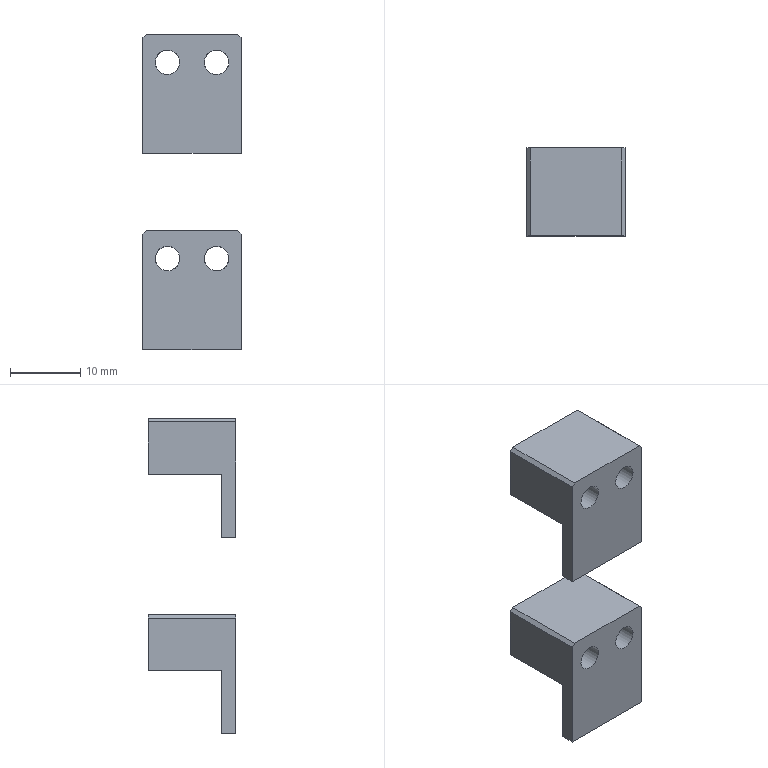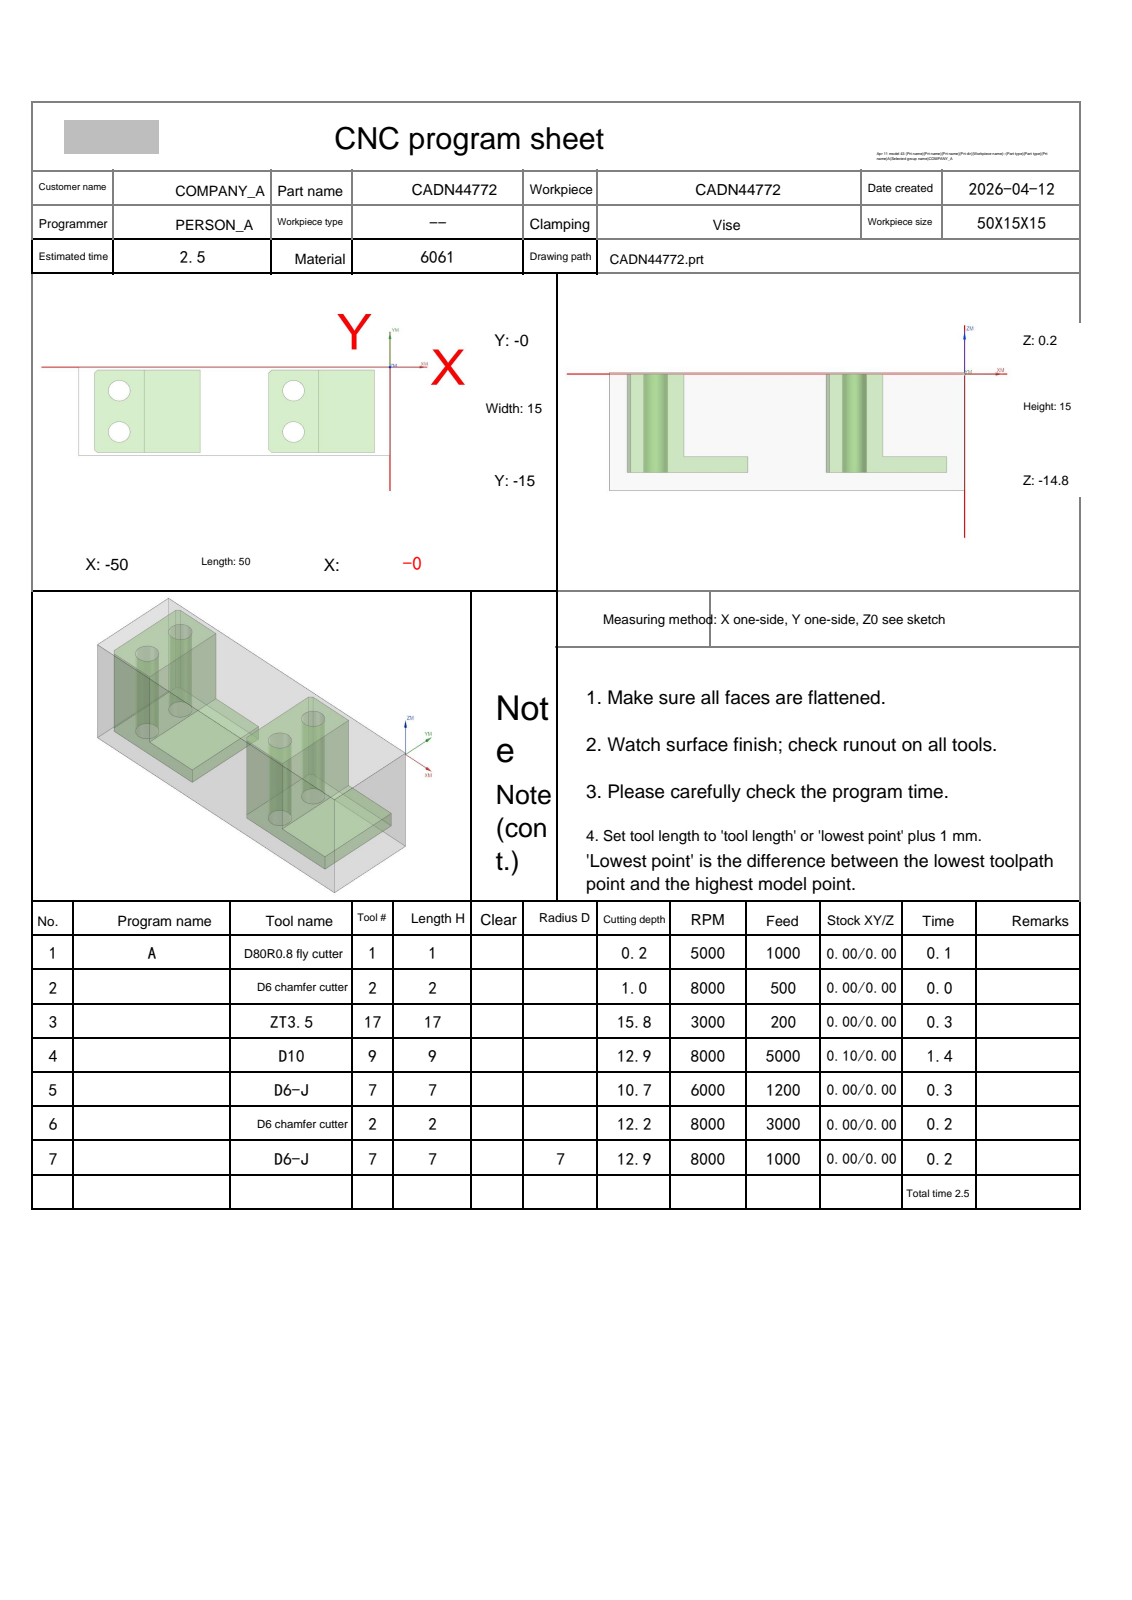NC program | NX | posted by the shop | part box 14 x 12.5 x 45 mm
Whole program:
%
O0001
(Machine time: 3.88 MIN)
(===Total Tool:5===)
(T1=D80R0.8 fly cutter D=80.  R=0.8  D-  H01 Z=-0.   )
(T2=D6 chamfer cutter   D=6.   R=0.   D-  H02 Z=-12.  )
(T17=ZT3.5  D=3.5  DR_a=118 D-  H17 Z=-15.55)
(T9=D10     D=10.  R=0.   D-  H09 Z=-12.7 )
(T7=D6-J    D=6.   R=0.   D7  H07 Z=-12.7 )
G80 G90 G17 G49 G40
G91 G28 Z0
M01
N1 T01 M06
(D80R0.8 fly cutter  D=80. R=0.8 H=01 ce=0.00 di=0.00)
G00 G90 G54 X-92.5 Y-7.5 M03 S5000
G43 H01 Z20.
M08
Z2.
G01 Z0.0 F1000.
X-87.5
X37.5
X42.5
Z2.
G00 Z20.
G91 G28 Z0.0
M05
M09
G91 G28 Z0.0
M01
N2 T02 M06
(D6 chamfer cutter  D=6. R=0. H=02 ce=0.00 di=0.00)
G00 G90 G54 X-43.5 Y-4. M03 S8000
G43 H02 Z20.
M08
G98 G81 X-43.5 Y-4. Z-.8 R1. F500.
Y-11.
X-15.5
Y-4.
G80
G00 Z20.
G91 G28 Z0.0
M05
M09
G91 G28 Z0.0
M01
N3 T17 M06
(ZT3.5 D=3.5 DR_a=118 H=17)
G00 G90 G54 X-43.5 Y-4. M03 S3000
G43 H17 Z20.
M08
G98 G83 X-43.5 Y-4. Z-15.552 R1. F200. Q3.
Y-11.
X-15.5
Y-4.
G80
G00 Z20.
G91 G28 Z0.0
M05
M09
G91 G28 Z0.0
M01
N4 T09 M06
(D10  D=10. R=0. H=09 ce=0.10 di=0.00)
G00 G90 G54 X-10.75 Y4.6 M03 S8000
G43 H09 Z20.
M08
Z.5
G01 X-2.5 Z.431 F5000.
G02 X2.6 Y-.5 Z.365 I0.0 J-5.1
G01 Y-14.5 Z.249
G02 X-2.5 Y-19.6 Z.182 I-5.1 J0.0
G01 X-19. Z.045
G02 X-22.606 Y-18.106 Z.012 I0.0 J5.1
G01 X-23.106 Y-17.606 Z.006
G02 X-24.6 Y-14. Z-.027 I3.606 J3.606
G01 Y-1. Z-.135
G02 X-23.106 Y2.606 Z-.169 I5.1 J0.0
G01 X-22.606 Y3.106 Z-.175
G02 X-19. Y4.6 Z-.208 I3.606 J-3.606
G01 X-2.5 Z-.345
G02 X2.6 Y-.5 Z-.412 I0.0 J-5.1
G01 Y-14.5 Z-.528
G02 X-2.5 Y-19.6 Z-.594 I-5.1 J0.0
G01 X-19. Z-.732
G02 X-22.606 Y-18.106 Z-.765 I0.0 J5.1
G01 X-23.106 Y-17.606 Z-.771
G02 X-24.6 Y-14. Z-.804 I3.606 J3.606
G01 Y-1. Z-.912
G02 X-23.106 Y2.606 Z-.945 I5.1 J0.0
G01 X-22.606 Y3.106 Z-.951
G02 X-19. Y4.6 Z-.984 I3.606 J-3.606
G01 X-2.5 Z-1.121
G02 X2.6 Y-.5 Z-1.188 I0.0 J-5.1
G01 Y-14.5 Z-1.304
G02 X-2.5 Y-19.6 Z-1.371 I-5.1 J0.0
G01 X-19. Z-1.508
G02 X-22.606 Y-18.106 Z-1.541 I0.0 J5.1
G01 X-23.106 Y-17.606 Z-1.547
G02 X-24.6 Y-14. Z-1.58 I3.606 J3.606
G01 Y-1. Z-1.688
G02 X-23.106 Y2.606 Z-1.722 I5.1 J0.0
G01 X-22.606 Y3.106 Z-1.728
G02 X-19. Y4.6 Z-1.761 I3.606 J-3.606
G01 X-2.5 Z-1.898
G02 X2.6 Y-.5 Z-1.965 I0.0 J-5.1
G01 Y-14.5 Z-2.081
G02 X-2.5 Y-19.6 Z-2.147 I-5.1 J0.0
G01 X-19. Z-2.284
G02 X-22.606 Y-18.106 Z-2.318 I0.0 J5.1
G01 X-23.106 Y-17.606 Z-2.324
G02 X-24.6 Y-14. Z-2.357 I3.606 J3.606
G01 Y-1. Z-2.465
G02 X-23.106 Y2.606 Z-2.498 I5.1 J0.0
G01 X-22.606 Y3.106 Z-2.504
G02 X-19. Y4.6 Z-2.537 I3.606 J-3.606
G01 X-2.5 Z-2.674
G02 X2.6 Y-.5 Z-2.741 I0.0 J-5.1
G01 Y-14.5 Z-2.857
G02 X-2.5 Y-19.6 Z-2.924 I-5.1 J0.0
G01 X-19. Z-3.061
G02 X-22.606 Y-18.106 Z-3.094 I0.0 J5.1
G01 X-23.106 Y-17.606 Z-3.1
G02 X-24.6 Y-14. Z-3.133 I3.606 J3.606
G01 Y-1. Z-3.241
G02 X-23.106 Y2.606 Z-3.275 I5.1 J0.0
G01 X-22.606 Y3.106 Z-3.281
G02 X-19. Y4.6 Z-3.314 I3.606 J-3.606
G01 X-2.5 Z-3.451
G02 X2.6 Y-.5 Z-3.517 I0.0 J-5.1
G01 Y-14.5 Z-3.634
G02 X-2.5 Y-19.6 Z-3.7 I-5.1 J0.0
G01 X-19. Z-3.837
G02 X-22.606 Y-18.106 Z-3.871 I0.0 J5.1
G01 X-23.106 Y-17.606 Z-3.877
G02 X-24.6 Y-14. Z-3.91 I3.606 J3.606
G01 Y-1. Z-4.018
G02 X-23.106 Y2.606 Z-4.051 I5.1 J0.0
G01 X-22.606 Y3.106 Z-4.057
G02 X-19. Y4.6 Z-4.09 I3.606 J-3.606
G01 X-2.5 Z-4.227
G02 X2.6 Y-.5 Z-4.294 I0.0 J-5.1
G01 Y-14.5 Z-4.41
G02 X-2.5 Y-19.6 Z-4.477 I-5.1 J0.0
G01 X-19. Z-4.614
G02 X-22.606 Y-18.106 Z-4.647 I0.0 J5.1
G01 X-23.106 Y-17.606 Z-4.653
G02 X-24.6 Y-14. Z-4.686 I3.606 J3.606
G01 Y-1. Z-4.794
G02 X-23.106 Y2.606 Z-4.828 I5.1 J0.0
G01 X-22.606 Y3.106 Z-4.833
G02 X-19. Y4.6 Z-4.867 I3.606 J-3.606
G01 X-2.5 Z-5.004
G02 X2.6 Y-.5 Z-5.07 I0.0 J-5.1
G01 Y-14.5 Z-5.187
G02 X-2.5 Y-19.6 Z-5.253 I-5.1 J0.0
G01 X-19. Z-5.39
G02 X-22.606 Y-18.106 Z-5.424 I0.0 J5.1
G01 X-23.106 Y-17.606 Z-5.43
G02 X-24.6 Y-14. Z-5.463 I3.606 J3.606
G01 Y-1. Z-5.571
G02 X-23.106 Y2.606 Z-5.604 I5.1 J0.0
G01 X-22.606 Y3.106 Z-5.61
G02 X-19. Y4.6 Z-5.643 I3.606 J-3.606
G01 X-2.5 Z-5.78
G02 X2.6 Y-.5 Z-5.847 I0.0 J-5.1
G01 Y-14.5 Z-5.963
G02 X-2.5 Y-19.6 Z-6.03 I-5.1 J0.0
G01 X-19. Z-6.167
G02 X-22.606 Y-18.106 Z-6.2 I0.0 J5.1
G01 X-23.106 Y-17.606 Z-6.206
G02 X-24.6 Y-14. Z-6.239 I3.606 J3.606
G01 Y-1. Z-6.347
G02 X-23.106 Y2.606 Z-6.381 I5.1 J0.0
G01 X-22.606 Y3.106 Z-6.386
G02 X-19. Y4.6 Z-6.42 I3.606 J-3.606
G01 X-2.5 Z-6.557
G02 X2.6 Y-.5 Z-6.623 I0.0 J-5.1
G01 Y-14.5 Z-6.74
G02 X-2.5 Y-19.6 Z-6.806 I-5.1 J0.0
G01 X-19. Z-6.943
G02 X-22.606 Y-18.106 Z-6.977 I0.0 J5.1
G01 X-23.106 Y-17.606 Z-6.982
G02 X-24.6 Y-14. Z-7.016 I3.606 J3.606
G01 Y-1. Z-7.124
G02 X-23.106 Y2.606 Z-7.157 I5.1 J0.0
G01 X-22.606 Y3.106 Z-7.163
G02 X-19. Y4.6 Z-7.196 I3.606 J-3.606
G01 X-2.5 Z-7.333
G02 X2.6 Y-.5 Z-7.4 I0.0 J-5.1
G01 Y-14.5 Z-7.516
G02 X-2.5 Y-19.6 Z-7.583 I-5.1 J0.0
G01 X-19. Z-7.72
G02 X-22.606 Y-18.106 Z-7.753 I0.0 J5.1
G01 X-23.106 Y-17.606 Z-7.759
G02 X-24.6 Y-14. Z-7.792 I3.606 J3.606
G01 Y-1. Z-7.9
G02 X-23.106 Y2.606 Z-7.933 I5.1 J0.0
G01 X-22.606 Y3.106 Z-7.939
G02 X-19. Y4.6 Z-7.973 I3.606 J-3.606
G01 X-2.5 Z-8.11
G02 X2.6 Y-.5 Z-8.176 I0.0 J-5.1
G01 Y-14.5 Z-8.293
G02 X-2.5 Y-19.6 Z-8.359 I-5.1 J0.0
G01 X-19. Z-8.496
G02 X-22.606 Y-18.106 Z-8.53 I0.0 J5.1
G01 X-23.106 Y-17.606 Z-8.535
G02 X-24.6 Y-14. Z-8.569 I3.606 J3.606
G01 Y-1. Z-8.677
G02 X-23.106 Y2.606 Z-8.71 I5.1 J0.0
G01 X-22.606 Y3.106 Z-8.716
G02 X-19. Y4.6 Z-8.749 I3.606 J-3.606
G01 X-2.5 Z-8.886
G02 X2.6 Y-.5 Z-8.953 I0.0 J-5.1
G01 Y-14.5 Z-9.069
G02 X-2.5 Y-19.6 Z-9.136 I-5.1 J0.0
G01 X-19. Z-9.273
G02 X-22.606 Y-18.106 Z-9.306 I0.0 J5.1
G01 X-23.106 Y-17.606 Z-9.312
G02 X-24.6 Y-14. Z-9.345 I3.606 J3.606
G01 Y-1. Z-9.453
G02 X-23.106 Y2.606 Z-9.486 I5.1 J0.0
G01 X-22.606 Y3.106 Z-9.492
G02 X-19. Y4.6 Z-9.526 I3.606 J-3.606
G01 X-2.5 Z-9.663
G02 X2.6 Y-.5 Z-9.729 I0.0 J-5.1
G01 Y-14.5 Z-9.846
G02 X-2.5 Y-19.6 Z-9.912 I-5.1 J0.0
G01 X-19. Z-10.049
G02 X-22.606 Y-18.106 Z-10.082 I0.0 J5.1
G01 X-23.106 Y-17.606 Z-10.088
G02 X-24.6 Y-14. Z-10.122 I3.606 J3.606
G01 Y-1. Z-10.23
G02 X-23.106 Y2.606 Z-10.263 I5.1 J0.0
G01 X-22.606 Y3.106 Z-10.269
G02 X-19. Y4.6 Z-10.302 I3.606 J-3.606
G01 X-2.5 Z-10.439
G02 X2.6 Y-.5 Z-10.506 I0.0 J-5.1
G01 Y-14.5 Z-10.622
G02 X-2.5 Y-19.6 Z-10.689 I-5.1 J0.0
G01 X-19. Z-10.826
G02 X-22.606 Y-18.106 Z-10.859 I0.0 J5.1
G01 X-23.106 Y-17.606 Z-10.865
G02 X-24.6 Y-14. Z-10.898 I3.606 J3.606
G01 Y-1. Z-11.006
G02 X-23.106 Y2.606 Z-11.039 I5.1 J0.0
G01 X-22.606 Y3.106 Z-11.045
G02 X-19. Y4.6 Z-11.079 I3.606 J-3.606
G01 X-2.5 Z-11.216
G02 X2.6 Y-.5 Z-11.282 I0.0 J-5.1
G01 Y-14.5 Z-11.398
G02 X-2.5 Y-19.6 Z-11.465 I-5.1 J0.0
G01 X-19. Z-11.602
G02 X-22.606 Y-18.106 Z-11.635 I0.0 J5.1
G01 X-23.106 Y-17.606 Z-11.641
G02 X-24.6 Y-14. Z-11.675 I3.606 J3.606
G01 Y-1. Z-11.783
G02 X-23.106 Y2.606 Z-11.816 I5.1 J0.0
G01 X-22.606 Y3.106 Z-11.822
G02 X-19. Y4.6 Z-11.855 I3.606 J-3.606
G01 X-2.5 Z-11.992
G02 X2.6 Y-.5 Z-12.059 I0.0 J-5.1
G01 Y-14.5 Z-12.175
G02 X-2.5 Y-19.6 Z-12.242 I-5.1 J0.0
G01 X-19. Z-12.379
G02 X-22.606 Y-18.106 Z-12.412 I0.0 J5.1
G01 X-23.106 Y-17.606 Z-12.418
G02 X-24.6 Y-14. Z-12.451 I3.606 J3.606
G01 Y-1. Z-12.559
G02 X-23.106 Y2.606 Z-12.592 I5.1 J0.0
G01 X-22.606 Y3.106 Z-12.598
G02 X-19. Y4.6 Z-12.631 I3.606 J-3.606
G01 X-10.75 Z-12.7
X-2.5
G02 X2.6 Y-.5 I0.0 J-5.1
G01 Y-14.5
G02 X-2.5 Y-19.6 I-5.1 J0.0
G01 X-19.
G02 X-22.606 Y-18.106 I0.0 J5.1
G01 X-23.106 Y-17.606
G02 X-24.6 Y-14. I3.606 J3.606
G01 Y-1.
G02 X-23.106 Y2.606 I5.1 J0.0
G01 X-22.606 Y3.106
G02 X-19. Y4.6 I3.606 J-3.606
G01 X-10.75
X-10.25
Z-11.7
G00 Z20.
X-38.75
Z.5
G01 X-30.5 Z.431
G02 X-25.4 Y-.5 Z.365 I0.0 J-5.1
G01 Y-14.5 Z.249
G02 X-30.5 Y-19.6 Z.182 I-5.1 J0.0
G01 X-47. Z.045
G02 X-50.606 Y-18.106 Z.012 I0.0 J5.1
G01 X-51.106 Y-17.606 Z.006
G02 X-52.6 Y-14. Z-.027 I3.606 J3.606
G01 Y-1. Z-.135
G02 X-51.106 Y2.606 Z-.169 I5.1 J0.0
G01 X-50.606 Y3.106 Z-.175
G02 X-47. Y4.6 Z-.208 I3.606 J-3.606
G01 X-30.5 Z-.345
G02 X-25.4 Y-.5 Z-.412 I0.0 J-5.1
G01 Y-14.5 Z-.528
G02 X-30.5 Y-19.6 Z-.594 I-5.1 J0.0
G01 X-47. Z-.732
G02 X-50.606 Y-18.106 Z-.765 I0.0 J5.1
G01 X-51.106 Y-17.606 Z-.771
G02 X-52.6 Y-14. Z-.804 I3.606 J3.606
G01 Y-1. Z-.912
G02 X-51.106 Y2.606 Z-.945 I5.1 J0.0
G01 X-50.606 Y3.106 Z-.951
G02 X-47. Y4.6 Z-.984 I3.606 J-3.606
G01 X-30.5 Z-1.121
G02 X-25.4 Y-.5 Z-1.188 I0.0 J-5.1
G01 Y-14.5 Z-1.304
G02 X-30.5 Y-19.6 Z-1.371 I-5.1 J0.0
G01 X-47. Z-1.508
G02 X-50.606 Y-18.106 Z-1.541 I0.0 J5.1
G01 X-51.106 Y-17.606 Z-1.547
G02 X-52.6 Y-14. Z-1.58 I3.606 J3.606
G01 Y-1. Z-1.688
G02 X-51.106 Y2.606 Z-1.722 I5.1 J0.0
G01 X-50.606 Y3.106 Z-1.728
G02 X-47. Y4.6 Z-1.761 I3.606 J-3.606
G01 X-30.5 Z-1.898
G02 X-25.4 Y-.5 Z-1.965 I0.0 J-5.1
G01 Y-14.5 Z-2.081
G02 X-30.5 Y-19.6 Z-2.147 I-5.1 J0.0
G01 X-47. Z-2.284
G02 X-50.606 Y-18.106 Z-2.318 I0.0 J5.1
G01 X-51.106 Y-17.606 Z-2.324
G02 X-52.6 Y-14. Z-2.357 I3.606 J3.606
G01 Y-1. Z-2.465
G02 X-51.106 Y2.606 Z-2.498 I5.1 J0.0
G01 X-50.606 Y3.106 Z-2.504
G02 X-47. Y4.6 Z-2.537 I3.606 J-3.606
G01 X-30.5 Z-2.674
G02 X-25.4 Y-.5 Z-2.741 I0.0 J-5.1
G01 Y-14.5 Z-2.857
G02 X-30.5 Y-19.6 Z-2.924 I-5.1 J0.0
G01 X-47. Z-3.061
G02 X-50.606 Y-18.106 Z-3.094 I0.0 J5.1
G01 X-51.106 Y-17.606 Z-3.1
G02 X-52.6 Y-14. Z-3.133 I3.606 J3.606
G01 Y-1. Z-3.241
G02 X-51.106 Y2.606 Z-3.275 I5.1 J0.0
G01 X-50.606 Y3.106 Z-3.281
G02 X-47. Y4.6 Z-3.314 I3.606 J-3.606
G01 X-30.5 Z-3.451
G02 X-25.4 Y-.5 Z-3.517 I0.0 J-5.1
G01 Y-14.5 Z-3.634
G02 X-30.5 Y-19.6 Z-3.7 I-5.1 J0.0
G01 X-47. Z-3.837
G02 X-50.606 Y-18.106 Z-3.871 I0.0 J5.1
G01 X-51.106 Y-17.606 Z-3.877
G02 X-52.6 Y-14. Z-3.91 I3.606 J3.606
G01 Y-1. Z-4.018
G02 X-51.106 Y2.606 Z-4.051 I5.1 J0.0
G01 X-50.606 Y3.106 Z-4.057
G02 X-47. Y4.6 Z-4.09 I3.606 J-3.606
G01 X-30.5 Z-4.227
G02 X-25.4 Y-.5 Z-4.294 I0.0 J-5.1
G01 Y-14.5 Z-4.41
G02 X-30.5 Y-19.6 Z-4.477 I-5.1 J0.0
G01 X-47. Z-4.614
G02 X-50.606 Y-18.106 Z-4.647 I0.0 J5.1
G01 X-51.106 Y-17.606 Z-4.653
G02 X-52.6 Y-14. Z-4.686 I3.606 J3.606
G01 Y-1. Z-4.794
G02 X-51.106 Y2.606 Z-4.828 I5.1 J0.0
G01 X-50.606 Y3.106 Z-4.833
G02 X-47. Y4.6 Z-4.867 I3.606 J-3.606
G01 X-30.5 Z-5.004
G02 X-25.4 Y-.5 Z-5.07 I0.0 J-5.1
G01 Y-14.5 Z-5.187
G02 X-30.5 Y-19.6 Z-5.253 I-5.1 J0.0
G01 X-47. Z-5.39
G02 X-50.606 Y-18.106 Z-5.424 I0.0 J5.1
G01 X-51.106 Y-17.606 Z-5.43
G02 X-52.6 Y-14. Z-5.463 I3.606 J3.606
G01 Y-1. Z-5.571
G02 X-51.106 Y2.606 Z-5.604 I5.1 J0.0
G01 X-50.606 Y3.106 Z-5.61
G02 X-47. Y4.6 Z-5.643 I3.606 J-3.606
G01 X-30.5 Z-5.78
G02 X-25.4 Y-.5 Z-5.847 I0.0 J-5.1
G01 Y-14.5 Z-5.963
G02 X-30.5 Y-19.6 Z-6.03 I-5.1 J0.0
G01 X-47. Z-6.167
G02 X-50.606 Y-18.106 Z-6.2 I0.0 J5.1
G01 X-51.106 Y-17.606 Z-6.206
G02 X-52.6 Y-14. Z-6.239 I3.606 J3.606
G01 Y-1. Z-6.347
G02 X-51.106 Y2.606 Z-6.381 I5.1 J0.0
G01 X-50.606 Y3.106 Z-6.386
G02 X-47. Y4.6 Z-6.42 I3.606 J-3.606
G01 X-30.5 Z-6.557
G02 X-25.4 Y-.5 Z-6.623 I0.0 J-5.1
G01 Y-14.5 Z-6.74
G02 X-30.5 Y-19.6 Z-6.806 I-5.1 J0.0
G01 X-47. Z-6.943
G02 X-50.606 Y-18.106 Z-6.977 I0.0 J5.1
G01 X-51.106 Y-17.606 Z-6.982
G02 X-52.6 Y-14. Z-7.016 I3.606 J3.606
G01 Y-1. Z-7.124
G02 X-51.106 Y2.606 Z-7.157 I5.1 J0.0
G01 X-50.606 Y3.106 Z-7.163
G02 X-47. Y4.6 Z-7.196 I3.606 J-3.606
G01 X-30.5 Z-7.333
G02 X-25.4 Y-.5 Z-7.4 I0.0 J-5.1
G01 Y-14.5 Z-7.516
G02 X-30.5 Y-19.6 Z-7.583 I-5.1 J0.0
G01 X-47. Z-7.72
G02 X-50.606 Y-18.106 Z-7.753 I0.0 J5.1
G01 X-51.106 Y-17.606 Z-7.759
G02 X-52.6 Y-14. Z-7.792 I3.606 J3.606
G01 Y-1. Z-7.9
G02 X-51.106 Y2.606 Z-7.933 I5.1 J0.0
G01 X-50.606 Y3.106 Z-7.939
G02 X-47. Y4.6 Z-7.973 I3.606 J-3.606
G01 X-30.5 Z-8.11
G02 X-25.4 Y-.5 Z-8.176 I0.0 J-5.1
G01 Y-14.5 Z-8.293
G02 X-30.5 Y-19.6 Z-8.359 I-5.1 J0.0
G01 X-47. Z-8.496
G02 X-50.606 Y-18.106 Z-8.53 I0.0 J5.1
G01 X-51.106 Y-17.606 Z-8.535
G02 X-52.6 Y-14. Z-8.569 I3.606 J3.606
G01 Y-1. Z-8.677
G02 X-51.106 Y2.606 Z-8.71 I5.1 J0.0
G01 X-50.606 Y3.106 Z-8.716
G02 X-47. Y4.6 Z-8.749 I3.606 J-3.606
G01 X-30.5 Z-8.886
G02 X-25.4 Y-.5 Z-8.953 I0.0 J-5.1
G01 Y-14.5 Z-9.069
G02 X-30.5 Y-19.6 Z-9.136 I-5.1 J0.0
G01 X-47. Z-9.273
G02 X-50.606 Y-18.106 Z-9.306 I0.0 J5.1
G01 X-51.106 Y-17.606 Z-9.312
G02 X-52.6 Y-14. Z-9.345 I3.606 J3.606
G01 Y-1. Z-9.453
G02 X-51.106 Y2.606 Z-9.486 I5.1 J0.0
G01 X-50.606 Y3.106 Z-9.492
G02 X-47. Y4.6 Z-9.526 I3.606 J-3.606
G01 X-30.5 Z-9.663
G02 X-25.4 Y-.5 Z-9.729 I0.0 J-5.1
G01 Y-14.5 Z-9.846
G02 X-30.5 Y-19.6 Z-9.912 I-5.1 J0.0
G01 X-47. Z-10.049
G02 X-50.606 Y-18.106 Z-10.082 I0.0 J5.1
G01 X-51.106 Y-17.606 Z-10.088
G02 X-52.6 Y-14. Z-10.122 I3.606 J3.606
G01 Y-1. Z-10.23
G02 X-51.106 Y2.606 Z-10.263 I5.1 J0.0
G01 X-50.606 Y3.106 Z-10.269
G02 X-47. Y4.6 Z-10.302 I3.606 J-3.606
G01 X-30.5 Z-10.439
G02 X-25.4 Y-.5 Z-10.506 I0.0 J-5.1
G01 Y-14.5 Z-10.622
G02 X-30.5 Y-19.6 Z-10.689 I-5.1 J0.0
G01 X-47. Z-10.826
G02 X-50.606 Y-18.106 Z-10.859 I0.0 J5.1
G01 X-51.106 Y-17.606 Z-10.865
G02 X-52.6 Y-14. Z-10.898 I3.606 J3.606
G01 Y-1. Z-11.006
G02 X-51.106 Y2.606 Z-11.039 I5.1 J0.0
G01 X-50.606 Y3.106 Z-11.045
G02 X-47. Y4.6 Z-11.079 I3.606 J-3.606
G01 X-30.5 Z-11.216
G02 X-25.4 Y-.5 Z-11.282 I0.0 J-5.1
G01 Y-14.5 Z-11.398
G02 X-30.5 Y-19.6 Z-11.465 I-5.1 J0.0
G01 X-47. Z-11.602
G02 X-50.606 Y-18.106 Z-11.635 I0.0 J5.1
G01 X-51.106 Y-17.606 Z-11.641
G02 X-52.6 Y-14. Z-11.675 I3.606 J3.606
G01 Y-1. Z-11.783
G02 X-51.106 Y2.606 Z-11.816 I5.1 J0.0
G01 X-50.606 Y3.106 Z-11.822
G02 X-47. Y4.6 Z-11.855 I3.606 J-3.606
G01 X-30.5 Z-11.992
G02 X-25.4 Y-.5 Z-12.059 I0.0 J-5.1
G01 Y-14.5 Z-12.175
G02 X-30.5 Y-19.6 Z-12.242 I-5.1 J0.0
G01 X-47. Z-12.379
G02 X-50.606 Y-18.106 Z-12.412 I0.0 J5.1
G01 X-51.106 Y-17.606 Z-12.418
G02 X-52.6 Y-14. Z-12.451 I3.606 J3.606
G01 Y-1. Z-12.559
G02 X-51.106 Y2.606 Z-12.592 I5.1 J0.0
G01 X-50.606 Y3.106 Z-12.598
G02 X-47. Y4.6 Z-12.631 I3.606 J-3.606
G01 X-38.75 Z-12.7
X-30.5
G02 X-25.4 Y-.5 I0.0 J-5.1
G01 Y-14.5
G02 X-30.5 Y-19.6 I-5.1 J0.0
G01 X-47.
G02 X-50.606 Y-18.106 I0.0 J5.1
G01 X-51.106 Y-17.606
G02 X-52.6 Y-14. I3.606 J3.606
G01 Y-1.
G02 X-51.106 Y2.606 I5.1 J0.0
G01 X-50.606 Y3.106
G02 X-47. Y4.6 I3.606 J-3.606
G01 X-38.75
X-38.25
Z-11.7
G00 Z20.
G00 G90 X-28.198 Y-22.378 M03 S6000
Z20.
Z.005
G01 Z-.495 F3500.
X-29.5 Y-7.5
Y.5
X-34.4
Y-15.5
X-29.5
Y-7.5
Y-7.
Z.005
G00 Z.5
X-28.198 Y-22.378
Z-.49
G01 Z-.99
X-29.5 Y-7.5
Y.5
X-34.4
Y-15.5
X-29.5
Y-7.5
Y-7.
Z-.49
G00 Z.005
X-28.198 Y-22.378
Z-.986
G01 Z-1.486
X-29.5 Y-7.5
Y.5
X-34.4
Y-15.5
X-29.5
Y-7.5
Y-7.
Z-.986
G00 Z-.49
X-28.198 Y-22.378
Z-1.481
G01 Z-1.981
X-29.5 Y-7.5
Y.5
X-34.4
Y-15.5
X-29.5
Y-7.5
Y-7.
Z-1.481
G00 Z-.986
X-28.198 Y-22.378
Z-1.976
G01 Z-2.476
X-29.5 Y-7.5
Y.5
X-34.4
Y-15.5
X-29.5
Y-7.5
Y-7.
Z-1.976
G00 Z-1.481
X-28.198 Y-22.378
Z-2.471
G01 Z-2.971
X-29.5 Y-7.5
Y.5
X-34.4
Y-15.5
X-29.5
Y-7.5
Y-7.
Z-2.471
G00 Z-1.976
X-28.198 Y-22.378
Z-2.967
G01 Z-3.467
X-29.5 Y-7.5
Y.5
X-34.4
Y-15.5
X-29.5
Y-7.5
Y-7.
Z-2.967
G00 Z-2.471
X-28.198 Y-22.378
Z-3.462
G01 Z-3.962
X-29.5 Y-7.5
Y.5
X-34.4
Y-15.5
X-29.5
Y-7.5
Y-7.
Z-3.462
G00 Z-2.967
X-28.198 Y-22.378
Z-3.957
G01 Z-4.457
X-29.5 Y-7.5
Y.5
X-34.4
Y-15.5
X-29.5
Y-7.5
Y-7.
Z-3.957
G00 Z-3.462
X-28.198 Y-22.378
Z-4.452
G01 Z-4.952
X-29.5 Y-7.5
Y.5
X-34.4
Y-15.5
X-29.5
Y-7.5
Y-7.
Z-4.452
G00 Z-3.957
X-28.198 Y-22.378
Z-4.948
G01 Z-5.448
X-29.5 Y-7.5
Y.5
X-34.4
Y-15.5
X-29.5
Y-7.5
Y-7.
Z-4.948
G00 Z-4.452
X-28.198 Y-22.378
Z-5.443
G01 Z-5.943
X-29.5 Y-7.5
Y.5
X-34.4
Y-15.5
X-29.5
Y-7.5
Y-7.
Z-5.443
G00 Z-4.948
X-28.198 Y-22.378
Z-5.938
G01 Z-6.438
X-29.5 Y-7.5
Y.5
X-34.4
Y-15.5
X-29.5
Y-7.5
Y-7.
Z-5.938
G00 Z-5.443
X-28.198 Y-22.378
Z-6.433
G01 Z-6.933
X-29.5 Y-7.5
Y.5
X-34.4
Y-15.5
X-29.5
Y-7.5
Y-7.
Z-6.433
G00 Z-5.938
X-28.198 Y-22.378
Z-6.929
G01 Z-7.429
X-29.5 Y-7.5
Y.5
X-34.4
Y-15.5
X-29.5
Y-7.5
Y-7.
Z-6.929
G00 Z-6.433
X-28.198 Y-22.378
Z-7.424
G01 Z-7.924
X-29.5 Y-7.5
Y.5
X-34.4
Y-15.5
X-29.5
Y-7.5
Y-7.
Z-7.424
G00 Z-6.929
X-28.198 Y-22.378
Z-7.919
G01 Z-8.419
X-29.5 Y-7.5
Y.5
X-34.4
Y-15.5
X-29.5
Y-7.5
Y-7.
Z-7.919
G00 Z-7.424
X-28.198 Y-22.378
Z-8.414
G01 Z-8.914
X-29.5 Y-7.5
Y.5
X-34.4
Y-15.5
X-29.5
Y-7.5
Y-7.
Z-8.414
G00 Z-7.919
X-28.198 Y-22.378
Z-8.91
G01 Z-9.41
X-29.5 Y-7.5
Y.5
X-34.4
Y-15.5
X-29.5
Y-7.5
Y-7.
Z-8.91
G00 Z-8.414
X-28.198 Y-22.378
Z-9.405
G01 Z-9.905
X-29.5 Y-7.5
Y.5
X-34.4
Y-15.5
X-29.5
Y-7.5
Y-7.
Z-9.405
G00 Z-8.91
X-28.198 Y-22.378
Z-9.9
G01 Z-10.4
X-29.5 Y-7.5
Y.5
X-34.4
Y-15.5
X-29.5
Y-7.5
Y-7.
Z-9.9
G00 Z20.
X5.5 Y-7.5
Z.005
G01 Z-.495
X-1.5
Y.5
X-6.4
Y-15.5
X-1.5
Y-7.5
Y-7.
Z.005
G00 Z.5
X5.5 Y-7.5
Z-.49
G01 Z-.99
X-1.5
Y.5
X-6.4
Y-15.5
X-1.5
Y-7.5
Y-7.
Z-.49
G00 Z.005
X5.5 Y-7.5
Z-.986
G01 Z-1.486
X-1.5
Y.5
X-6.4
Y-15.5
X-1.5
Y-7.5
Y-7.
Z-.986
G00 Z-.49
X5.5 Y-7.5
Z-1.481
G01 Z-1.981
X-1.5
Y.5
X-6.4
Y-15.5
X-1.5
Y-7.5
Y-7.
Z-1.481
G00 Z-.986
X5.5 Y-7.5
Z-1.976
G01 Z-2.476
X-1.5
Y.5
X-6.4
Y-15.5
X-1.5
Y-7.5
Y-7.
Z-1.976
G00 Z-1.481
X5.5 Y-7.5
Z-2.471
G01 Z-2.971
X-1.5
Y.5
X-6.4
Y-15.5
X-1.5
Y-7.5
Y-7.
Z-2.471
G00 Z-1.976
X5.5 Y-7.5
Z-2.967
G01 Z-3.467
X-1.5
Y.5
X-6.4
Y-15.5
X-1.5
Y-7.5
Y-7.
Z-2.967
G00 Z-2.471
X5.5 Y-7.5
Z-3.462
G01 Z-3.962
X-1.5
Y.5
X-6.4
Y-15.5
X-1.5
Y-7.5
Y-7.
Z-3.462
G00 Z-2.967
X5.5 Y-7.5
Z-3.957
G01 Z-4.457
X-1.5
Y.5
X-6.4
Y-15.5
X-1.5
Y-7.5
Y-7.
Z-3.957
G00 Z-3.462
X5.5 Y-7.5
Z-4.452
G01 Z-4.952
X-1.5
Y.5
X-6.4
Y-15.5
X-1.5
Y-7.5
Y-7.
Z-4.452
G00 Z-3.957
X5.5 Y-7.5
Z-4.948
G01 Z-5.448
X-1.5
Y.5
X-6.4
Y-15.5
X-1.5
Y-7.5
Y-7.
Z-4.948
G00 Z-4.452
X5.5 Y-7.5
Z-5.443
G01 Z-5.943
X-1.5
Y.5
X-6.4
Y-15.5
X-1.5
Y-7.5
Y-7.
Z-5.443
G00 Z-4.948
X5.5 Y-7.5
Z-5.938
G01 Z-6.438
X-1.5
Y.5
X-6.4
Y-15.5
X-1.5
Y-7.5
Y-7.
Z-5.938
G00 Z-5.443
X5.5 Y-7.5
Z-6.433
G01 Z-6.933
X-1.5
Y.5
X-6.4
Y-15.5
X-1.5
Y-7.5
Y-7.
Z-6.433
G00 Z-5.938
X5.5 Y-7.5
Z-6.929
G01 Z-7.429
X-1.5
Y.5
X-6.4
Y-15.5
X-1.5
Y-7.5
Y-7.
Z-6.929
G00 Z-6.433
X5.5 Y-7.5
Z-7.424
G01 Z-7.924
X-1.5
Y.5
X-6.4
Y-15.5
X-1.5
Y-7.5
Y-7.
Z-7.424
G00 Z-6.929
X5.5 Y-7.5
Z-7.919
G01 Z-8.419
X-1.5
Y.5
X-6.4
Y-15.5
X-1.5
Y-7.5
Y-7.
Z-7.919
G00 Z-7.424
X5.5 Y-7.5
Z-8.414
G01 Z-8.914
X-1.5
Y.5
X-6.4
Y-15.5
X-1.5
Y-7.5
Y-7.
Z-8.414
G00 Z-7.919
X5.5 Y-7.5
Z-8.91
G01 Z-9.41
X-1.5
Y.5
X-6.4
Y-15.5
X-1.5
Y-7.5
Y-7.
Z-8.91
G00 Z-8.414
X5.5 Y-7.5
Z-9.405
G01 Z-9.905
X-1.5
Y.5
X-6.4
Y-15.5
X-1.5
Y-7.5
Y-7.
Z-9.405
G00 Z-8.91
X5.5 Y-7.5
Z-9.9
G01 Z-10.4
X-1.5
Y.5
X-6.4
Y-15.5
X-1.5
Y-7.5
Y-7.
Z-9.9
G00 Z20.
G91 G28 Z0.0
M05
M09
G91 G28 Z0.0
M01
N5 T07 M06
(D6-J  D=6. R=0. H=07 ce=0.30 di=0.00)
G00 G90 G54 X-25.013 Y-17.397 M03 S6000
G43 H07 Z20.
M08
Z-10.
G01 Z-10.5 F1200.
X-26.3 Y-7.5
X-29.9
Y-15.1
X-36.2
Y.1
X-29.9
Y-7.5
X-32.6
Y-12.4
X-33.5
Y-2.6
X-32.6
Y-7.5
Y-8.
X-29.
X-25.013 Y-17.397
Z-10.
G00 Z20.
X3.5 Y-7.5
Z-10.
G01 Z-10.5
X-1.9
Y-15.1
X-8.2
Y.1
X-1.9
Y-7.5
X-4.6
Y-12.4
X-5.5
Y-2.6
X-4.6
Y-7.5
Y-8.
X3.5
Z-10.
G00 Z20.
G00 G90 X-35.4 Y3.2 M03 S6000
Z20.
Z-4.748
G01 Z-5.248 F1200.
G41 D07
X-35.5
G03 X-36.5 Y2.2 I0.0 J-1.
G01 Y-17.2
G03 X-35.5 Y-18.2 I1. J0.0
G01 G40 X-35.4
Z-4.748
G00 Z20.
Y3.2
Z-9.995
G01 Z-10.495
G41 D07
X-35.5
G03 X-36.5 Y2.2 I0.0 J-1.
G01 Y-17.2
G03 X-35.5 Y-18.2 I1. J0.0
G01 G40 X-35.4
Z-9.995
G00 Z20.
X-7.4 Y3.2
Z-4.748
G01 Z-5.248
G41 D07
X-7.5
G03 X-8.5 Y2.2 I0.0 J-1.
G01 Y-17.2
G03 X-7.5 Y-18.2 I1. J0.0
G01 G40 X-7.4
Z-4.748
G00 Z20.
Y3.2
Z-9.995
G01 Z-10.495
G41 D07
X-7.5
G03 X-8.5 Y2.2 I0.0 J-1.
G01 Y-17.2
G03 X-7.5 Y-18.2 I1. J0.0
G01 G40 X-7.4
Z-9.995
G00 Z20.
G91 G28 Z0.0
M05
M09
G91 G28 Z0.0
M01
N6 T02 M06
(D6 chamfer cutter  D=6. R=0. H=02 ce=0.00 di=0.00)
G00 G90 G54 X-37.372 Y-7.25 M03 S8000
G43 H02 Z20.
M08
Z2.099
G01 Z-1.5 F3000.
G03 X-37.672 Y-7.17 I-.3 J-.52
X-38.192 Y-7.47 I0.0 J-.6
G01 X-38.2 Y-7.5
Y-14.5
G02 X-39.5 Y-15.8 I-1.3 J0.0
G01 X-47.
X-47.254 Y-15.775
X-47.497 Y-15.701
X-47.722 Y-15.581
X-47.919 Y-15.419
X-48.419 Y-14.919
X-48.581 Y-14.722
X-48.701 Y-14.497
X-48.775 Y-14.254
X-48.8 Y-14.
Y-1.
X-48.775 Y-.746
X-48.701 Y-.503
X-48.581 Y-.278
X-48.419 Y-.081
X-47.919 Y.419
X-47.722 Y.581
X-47.497 Y.701
X-47.254 Y.775
X-47. Y.8
X-39.5
G02 X-38.2 Y-.5 I0.0 J-1.3
G01 Y-7.5
X-38.192 Y-7.53
G03 X-37.672 Y-7.83 I.52 J.3
X-37.372 Y-7.75 I0.0 J.6
G01 Z2.099
G00 Z20.
X-21.628
Z2.099
G01 Z-1.5
G03 X-21.328 Y-7.83 I.3 J.52
X-20.808 Y-7.53 I0.0 J.6
G01 X-20.8 Y-7.5
Y-1.
X-20.775 Y-.746
X-20.701 Y-.503
X-20.581 Y-.278
X-20.419 Y-.081
X-19.919 Y.419
X-19.722 Y.581
X-19.497 Y.701
X-19.254 Y.775
X-19. Y.8
X-11.5
G02 X-10.2 Y-.5 I0.0 J-1.3
G01 Y-14.5
G02 X-11.5 Y-15.8 I-1.3 J0.0
G01 X-19.
X-19.254 Y-15.775
X-19.497 Y-15.701
X-19.722 Y-15.581
X-19.919 Y-15.419
X-20.419 Y-14.919
X-20.581 Y-14.722
X-20.701 Y-14.497
X-20.775 Y-14.254
X-20.8 Y-14.
Y-7.5
X-20.808 Y-7.47
G03 X-21.328 Y-7.17 I-.52 J-.3
X-21.628 Y-7.25 I0.0 J-.6
G01 Z2.099
G00 Z20.
X-36.445 Y1.628
Z1.755
G01 Z-12.
G03 X-36.525 Y1.328 I.52 J-.3
X-36.225 Y.808 I.6 J0.0
G01 X-36.195 Y.8
X-30.5
G02 X-29.2 Y-.5 I0.0 J-1.3
G01 Y-14.5
G02 X-30.5 Y-15.8 I-1.3 J0.0
G01 X-36.195
X-36.225 Y-15.808
G03 X-36.525 Y-16.328 I.3 J-.52
X-36.445 Y-16.628 I.6 J0.0
G01 Z1.755
G00 Z20.
X-8.445 Y1.628
Z1.755
G01 Z-12.
G03 X-8.525 Y1.328 I.52 J-.3
X-8.225 Y.808 I.6 J0.0
G01 X-8.195 Y.8
X-2.5
G02 X-1.2 Y-.5 I0.0 J-1.3
G01 Y-14.5
G02 X-2.5 Y-15.8 I-1.3 J0.0
G01 X-8.195
X-8.225 Y-15.808
G03 X-8.525 Y-16.328 I.3 J-.52
X-8.445 Y-16.628 I.6 J0.0
G01 Z1.755
G00 Z20.
G00 G90 X-43.5 Y-4. M03 S8000
Z20.
G98 G81 X-43.5 Y-4. Z-2.05 R3. F500.
Y-11.
X-15.5
Y-4.
G80
G00 Z20.
G91 G28 Z0.0
M05
M09
G91 G28 Z0.0
M01
N7 T07 M06
(D6-J  D=6. R=0. H=07 ce=0.00 di=0.00)
G00 G90 G54 X-29.483 Y-18.573 M03 S8000
G43 H07 Z20.
M08
Z-12.2
G01 Z-12.7 F1000.
G41 D07
X-29.508 Y-18.375
G03 X-30.5 Y-17.5 I-.992 J-.125
G01 X-47.
G02 X-49.121 Y-16.621 I0.0 J3.
G01 X-49.621 Y-16.121
G02 X-50.5 Y-14. I2.121 J2.121
G01 Y-1.
G02 X-49.621 Y1.121 I3. J0.0
G01 X-49.121 Y1.621
G02 X-47. Y2.5 I2.121 J-2.121
G01 X-30.5
G02 X-27.5 Y-.5 I0.0 J-3.
G01 Y-14.5
G02 X-30.5 Y-17.5 I-3. J0.0
G01 X-31.
G03 X-32. Y-18.5 I0.0 J-1.
G01 G40 Y-18.7
Z-12.2
G00 Z20.
X-1.483 Y-18.573
Z-12.2
G01 Z-12.7
G41 D07
X-1.508 Y-18.375
G03 X-2.5 Y-17.5 I-.992 J-.125
G01 X-19.
G02 X-21.121 Y-16.621 I0.0 J3.
G01 X-21.621 Y-16.121
G02 X-22.5 Y-14. I2.121 J2.121
G01 Y-1.
G02 X-21.621 Y1.121 I3. J0.0
G01 X-21.121 Y1.621
G02 X-19. Y2.5 I2.121 J-2.121
G01 X-2.5
G02 X.5 Y-.5 I0.0 J-3.
G01 Y-14.5
G02 X-2.5 Y-17.5 I-3. J0.0
G01 X-3.
G03 X-4. Y-18.5 I0.0 J-1.
G01 G40 Y-18.7
Z-12.2
G00 Z20.
M05
M09
G91 G28 Z0.0
G91 G28 Y0.0
M30
%